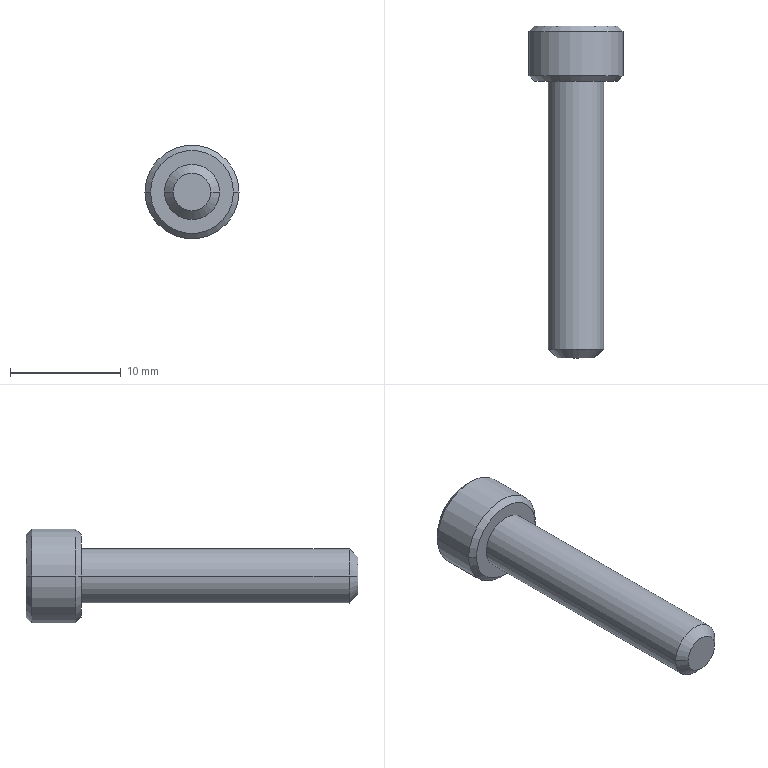Part | STEP file | BB62-M5-25L-1 | 1 solid | 27 faces | box 8.5 x 30 x 8.5 mm | volume 722.372 mm3 | plane 15 | cone 8 | cylinder 4 | commonest cylinder face diameters 5 x2 8.5 x2
STEP:
#1=CARTESIAN_POINT('',(0.,1.178,0.));
#2=VERTEX_POINT('',#1);
#3=CARTESIAN_POINT('',(2.29,2.5,0.));
#4=VERTEX_POINT('',#3);
#5=CARTESIAN_POINT('',(0.,1.178,0.));
#6=DIRECTION('',(0.866,0.5,0.));
#7=VECTOR('',#6,1000.);
#8=LINE('',#5,#7);
#9=EDGE_CURVE('',#2,#4,#8,.T.);
#10=ORIENTED_EDGE('',*,*,#9,.F.);
#11=CARTESIAN_POINT('',(-2.29,2.5,0.));
#12=VERTEX_POINT('',#11);
#13=CARTESIAN_POINT('',(0.,1.178,0.));
#14=DIRECTION('',(-0.866,0.5,0.));
#15=VECTOR('',#14,1000.);
#16=LINE('',#13,#15);
#17=EDGE_CURVE('',#2,#12,#16,.T.);
#18=ORIENTED_EDGE('',*,*,#17,.T.);
#19=CARTESIAN_POINT('',(-1.983,2.5,1.145));
#20=VERTEX_POINT('',#19);
#21=CARTESIAN_POINT('',(0.,2.5,0.));
#22=DIRECTION('',(0.,-1.,0.));
#23=DIRECTION('',(-1.,0.,0.));
#24=AXIS2_PLACEMENT_3D('',#21,#22,#23);
#25=CIRCLE('',#24,2.29);
#26=EDGE_CURVE('',#20,#12,#25,.T.);
#27=ORIENTED_EDGE('',*,*,#26,.F.);
#28=CARTESIAN_POINT('',(0.,2.5,2.29));
#29=VERTEX_POINT('',#28);
#30=CARTESIAN_POINT('',(0.,2.5,0.));
#31=DIRECTION('',(0.,-1.,0.));
#32=DIRECTION('',(-1.,0.,0.));
#33=AXIS2_PLACEMENT_3D('',#30,#31,#32);
#34=CIRCLE('',#33,2.29);
#35=EDGE_CURVE('',#29,#20,#34,.T.);
#36=ORIENTED_EDGE('',*,*,#35,.F.);
#37=CARTESIAN_POINT('',(1.983,2.5,1.145));
#38=VERTEX_POINT('',#37);
#39=CARTESIAN_POINT('',(0.,2.5,0.));
#40=DIRECTION('',(0.,-1.,0.));
#41=DIRECTION('',(-1.,0.,0.));
#42=AXIS2_PLACEMENT_3D('',#39,#40,#41);
#43=CIRCLE('',#42,2.29);
#44=EDGE_CURVE('',#38,#29,#43,.T.);
#45=ORIENTED_EDGE('',*,*,#44,.F.);
#46=CARTESIAN_POINT('',(0.,2.5,0.));
#47=DIRECTION('',(0.,-1.,0.));
#48=DIRECTION('',(-1.,0.,0.));
#49=AXIS2_PLACEMENT_3D('',#46,#47,#48);
#50=CIRCLE('',#49,2.29);
#51=EDGE_CURVE('',#4,#38,#50,.T.);
#52=ORIENTED_EDGE('',*,*,#51,.F.);
#53=EDGE_LOOP('',(#10,#18,#27,#36,#45,#52));
#54=FACE_OUTER_BOUND('',#53,.T.);
#55=CARTESIAN_POINT('',(0.,1001.178,0.));
#56=DIRECTION('',(0.,1.,0.));
#57=DIRECTION('',(1.,0.,0.));
#58=AXIS2_PLACEMENT_3D('',#55,#56,#57);
#59=CONICAL_SURFACE('',#58,1732.051,1.047);
#60=ADVANCED_FACE('',(#54),#59,.F.);
#61=CARTESIAN_POINT('',(1.7,-25.,0.));
#62=VERTEX_POINT('',#61);
#63=CARTESIAN_POINT('',(-1.7,-25.,0.));
#64=VERTEX_POINT('',#63);
#65=CARTESIAN_POINT('',(0.,-25.,0.));
#66=DIRECTION('',(0.,1.,0.));
#67=DIRECTION('',(1.,0.,0.));
#68=AXIS2_PLACEMENT_3D('',#65,#66,#67);
#69=CIRCLE('',#68,1.7);
#70=EDGE_CURVE('',#62,#64,#69,.T.);
#71=ORIENTED_EDGE('',*,*,#70,.T.);
#72=CARTESIAN_POINT('',(-2.5,-24.2,0.));
#73=VERTEX_POINT('',#72);
#74=CARTESIAN_POINT('',(-1.7,-25.,0.));
#75=DIRECTION('',(-0.7071,0.7071,0.));
#76=VECTOR('',#75,1000.);
#77=LINE('',#74,#76);
#78=EDGE_CURVE('',#64,#73,#77,.T.);
#79=ORIENTED_EDGE('',*,*,#78,.T.);
#80=CARTESIAN_POINT('',(2.5,-24.2,0.));
#81=VERTEX_POINT('',#80);
#82=CARTESIAN_POINT('',(0.,-24.2,0.));
#83=DIRECTION('',(0.,-1.,0.));
#84=DIRECTION('',(-1.,0.,0.));
#85=AXIS2_PLACEMENT_3D('',#82,#83,#84);
#86=CIRCLE('',#85,2.5);
#87=EDGE_CURVE('',#73,#81,#86,.T.);
#88=ORIENTED_EDGE('',*,*,#87,.T.);
#89=CARTESIAN_POINT('',(1.7,-25.,0.));
#90=DIRECTION('',(0.7071,0.7071,0.));
#91=VECTOR('',#90,1000.);
#92=LINE('',#89,#91);
#93=EDGE_CURVE('',#62,#81,#92,.T.);
#94=ORIENTED_EDGE('',*,*,#93,.F.);
#95=EDGE_LOOP('',(#71,#79,#88,#94));
#96=FACE_OUTER_BOUND('',#95,.T.);
#97=CARTESIAN_POINT('',(0.,-25.,0.));
#98=DIRECTION('',(0.,1.,0.));
#99=DIRECTION('',(1.,0.,0.));
#100=AXIS2_PLACEMENT_3D('',#97,#98,#99);
#101=CONICAL_SURFACE('',#100,1.7,0.7854);
#102=ADVANCED_FACE('',(#96),#101,.T.);
#103=ORIENTED_EDGE('',*,*,#87,.F.);
#104=CARTESIAN_POINT('',(-2.5,0.,0.));
#105=VERTEX_POINT('',#104);
#106=CARTESIAN_POINT('',(-2.5,-24.2,0.));
#107=DIRECTION('',(0.,1.,0.));
#108=VECTOR('',#107,1000.);
#109=LINE('',#106,#108);
#110=EDGE_CURVE('',#73,#105,#109,.T.);
#111=ORIENTED_EDGE('',*,*,#110,.T.);
#112=CARTESIAN_POINT('',(2.5,0.,0.));
#113=VERTEX_POINT('',#112);
#114=CARTESIAN_POINT('',(0.,0.,0.));
#115=DIRECTION('',(0.,-1.,0.));
#116=DIRECTION('',(-1.,0.,0.));
#117=AXIS2_PLACEMENT_3D('',#114,#115,#116);
#118=CIRCLE('',#117,2.5);
#119=EDGE_CURVE('',#105,#113,#118,.T.);
#120=ORIENTED_EDGE('',*,*,#119,.T.);
#121=CARTESIAN_POINT('',(2.5,-24.2,0.));
#122=DIRECTION('',(0.,1.,0.));
#123=VECTOR('',#122,1000.);
#124=LINE('',#121,#123);
#125=EDGE_CURVE('',#81,#113,#124,.T.);
#126=ORIENTED_EDGE('',*,*,#125,.F.);
#127=EDGE_LOOP('',(#103,#111,#120,#126));
#128=FACE_OUTER_BOUND('',#127,.T.);
#129=CARTESIAN_POINT('',(0.,-24.2,0.));
#130=DIRECTION('',(0.,1.,0.));
#131=DIRECTION('',(1.,0.,0.));
#132=AXIS2_PLACEMENT_3D('',#129,#130,#131);
#133=CYLINDRICAL_SURFACE('',#132,2.5);
#134=ADVANCED_FACE('',(#128),#133,.T.);
#135=CARTESIAN_POINT('',(-3.75,5.,0.));
#136=VERTEX_POINT('',#135);
#137=CARTESIAN_POINT('',(3.75,5.,0.));
#138=VERTEX_POINT('',#137);
#139=CARTESIAN_POINT('',(0.,5.,0.));
#140=DIRECTION('',(0.,-1.,0.));
#141=DIRECTION('',(-1.,0.,0.));
#142=AXIS2_PLACEMENT_3D('',#139,#140,#141);
#143=CIRCLE('',#142,3.75);
#144=EDGE_CURVE('',#136,#138,#143,.T.);
#145=ORIENTED_EDGE('',*,*,#144,.T.);
#146=CARTESIAN_POINT('',(4.25,4.5,0.));
#147=VERTEX_POINT('',#146);
#148=CARTESIAN_POINT('',(4.25,4.5,0.));
#149=DIRECTION('',(0.7071,-0.7071,0.));
#150=VECTOR('',#149,1000.);
#151=LINE('',#148,#150);
#152=EDGE_CURVE('',#138,#147,#151,.T.);
#153=ORIENTED_EDGE('',*,*,#152,.T.);
#154=CARTESIAN_POINT('',(-4.25,4.5,0.));
#155=VERTEX_POINT('',#154);
#156=CARTESIAN_POINT('',(0.,4.5,0.));
#157=DIRECTION('',(0.,-1.,0.));
#158=DIRECTION('',(-1.,0.,0.));
#159=AXIS2_PLACEMENT_3D('',#156,#157,#158);
#160=CIRCLE('',#159,4.25);
#161=EDGE_CURVE('',#155,#147,#160,.T.);
#162=ORIENTED_EDGE('',*,*,#161,.F.);
#163=CARTESIAN_POINT('',(-4.25,4.5,0.));
#164=DIRECTION('',(-0.7071,-0.7071,0.));
#165=VECTOR('',#164,1000.);
#166=LINE('',#163,#165);
#167=EDGE_CURVE('',#136,#155,#166,.T.);
#168=ORIENTED_EDGE('',*,*,#167,.F.);
#169=EDGE_LOOP('',(#145,#153,#162,#168));
#170=FACE_OUTER_BOUND('',#169,.T.);
#171=CARTESIAN_POINT('',(0.,4.5,0.));
#172=DIRECTION('',(0.,-1.,0.));
#173=DIRECTION('',(-1.,0.,0.));
#174=AXIS2_PLACEMENT_3D('',#171,#172,#173);
#175=CONICAL_SURFACE('',#174,4.25,0.7854);
#176=ADVANCED_FACE('',(#170),#175,.T.);
#177=ORIENTED_EDGE('',*,*,#161,.T.);
#178=CARTESIAN_POINT('',(4.25,0.5,0.));
#179=VERTEX_POINT('',#178);
#180=CARTESIAN_POINT('',(4.25,1.62,0.));
#181=DIRECTION('',(0.,-1.,0.));
#182=VECTOR('',#181,1000.);
#183=LINE('',#180,#182);
#184=EDGE_CURVE('',#147,#179,#183,.T.);
#185=ORIENTED_EDGE('',*,*,#184,.T.);
#186=CARTESIAN_POINT('',(-4.25,0.5,0.));
#187=VERTEX_POINT('',#186);
#188=CARTESIAN_POINT('',(0.,0.5,0.));
#189=DIRECTION('',(0.,-1.,0.));
#190=DIRECTION('',(-1.,0.,0.));
#191=AXIS2_PLACEMENT_3D('',#188,#189,#190);
#192=CIRCLE('',#191,4.25);
#193=EDGE_CURVE('',#187,#179,#192,.T.);
#194=ORIENTED_EDGE('',*,*,#193,.F.);
#195=CARTESIAN_POINT('',(-4.25,1.62,0.));
#196=DIRECTION('',(0.,-1.,0.));
#197=VECTOR('',#196,1000.);
#198=LINE('',#195,#197);
#199=EDGE_CURVE('',#155,#187,#198,.T.);
#200=ORIENTED_EDGE('',*,*,#199,.F.);
#201=EDGE_LOOP('',(#177,#185,#194,#200));
#202=FACE_OUTER_BOUND('',#201,.T.);
#203=CARTESIAN_POINT('',(0.,1.62,0.));
#204=DIRECTION('',(0.,-1.,0.));
#205=DIRECTION('',(-1.,0.,0.));
#206=AXIS2_PLACEMENT_3D('',#203,#204,#205);
#207=CYLINDRICAL_SURFACE('',#206,4.25);
#208=ADVANCED_FACE('',(#202),#207,.T.);
#209=CARTESIAN_POINT('',(-3.75,0.,0.));
#210=VERTEX_POINT('',#209);
#211=CARTESIAN_POINT('',(3.75,0.,0.));
#212=VERTEX_POINT('',#211);
#213=CARTESIAN_POINT('',(0.,0.,0.));
#214=DIRECTION('',(0.,-1.,0.));
#215=DIRECTION('',(-1.,0.,0.));
#216=AXIS2_PLACEMENT_3D('',#213,#214,#215);
#217=CIRCLE('',#216,3.75);
#218=EDGE_CURVE('',#210,#212,#217,.T.);
#219=ORIENTED_EDGE('',*,*,#218,.F.);
#220=CARTESIAN_POINT('',(-3.75,0.,0.));
#221=DIRECTION('',(-0.7071,0.7071,0.));
#222=VECTOR('',#221,1000.);
#223=LINE('',#220,#222);
#224=EDGE_CURVE('',#210,#187,#223,.T.);
#225=ORIENTED_EDGE('',*,*,#224,.T.);
#226=ORIENTED_EDGE('',*,*,#193,.T.);
#227=CARTESIAN_POINT('',(3.75,0.,0.));
#228=DIRECTION('',(0.7071,0.7071,0.));
#229=VECTOR('',#228,1000.);
#230=LINE('',#227,#229);
#231=EDGE_CURVE('',#212,#179,#230,.T.);
#232=ORIENTED_EDGE('',*,*,#231,.F.);
#233=EDGE_LOOP('',(#219,#225,#226,#232));
#234=FACE_OUTER_BOUND('',#233,.T.);
#235=CARTESIAN_POINT('',(0.,0.,0.));
#236=DIRECTION('',(0.,1.,0.));
#237=DIRECTION('',(1.,0.,0.));
#238=AXIS2_PLACEMENT_3D('',#235,#236,#237);
#239=CONICAL_SURFACE('',#238,3.75,0.7854);
#240=ADVANCED_FACE('',(#234),#239,.T.);
#241=ORIENTED_EDGE('',*,*,#144,.F.);
#242=CARTESIAN_POINT('',(0.,5.,0.));
#243=DIRECTION('',(0.,-1.,0.));
#244=DIRECTION('',(-1.,0.,0.));
#245=AXIS2_PLACEMENT_3D('',#242,#243,#244);
#246=CIRCLE('',#245,3.75);
#247=EDGE_CURVE('',#138,#136,#246,.T.);
#248=ORIENTED_EDGE('',*,*,#247,.F.);
#249=EDGE_LOOP('',(#241,#248));
#250=FACE_OUTER_BOUND('',#249,.T.);
#251=CARTESIAN_POINT('',(0.,5.,-2.29));
#252=VERTEX_POINT('',#251);
#253=CARTESIAN_POINT('',(-1.983,5.,-1.145));
#254=VERTEX_POINT('',#253);
#255=CARTESIAN_POINT('',(0.,5.,-2.29));
#256=DIRECTION('',(-0.866,0.,0.5));
#257=VECTOR('',#256,1000.);
#258=LINE('',#255,#257);
#259=EDGE_CURVE('',#252,#254,#258,.T.);
#260=ORIENTED_EDGE('',*,*,#259,.F.);
#261=CARTESIAN_POINT('',(1.983,5.,-1.145));
#262=VERTEX_POINT('',#261);
#263=CARTESIAN_POINT('',(1.983,5.,-1.145));
#264=DIRECTION('',(-0.866,0.,-0.5));
#265=VECTOR('',#264,1000.);
#266=LINE('',#263,#265);
#267=EDGE_CURVE('',#262,#252,#266,.T.);
#268=ORIENTED_EDGE('',*,*,#267,.F.);
#269=CARTESIAN_POINT('',(1.983,5.,1.145));
#270=VERTEX_POINT('',#269);
#271=CARTESIAN_POINT('',(1.983,5.,1.145));
#272=DIRECTION('',(0.,0.,-1.));
#273=VECTOR('',#272,1000.);
#274=LINE('',#271,#273);
#275=EDGE_CURVE('',#270,#262,#274,.T.);
#276=ORIENTED_EDGE('',*,*,#275,.F.);
#277=CARTESIAN_POINT('',(0.,5.,2.29));
#278=VERTEX_POINT('',#277);
#279=CARTESIAN_POINT('',(0.,5.,2.29));
#280=DIRECTION('',(0.866,0.,-0.5));
#281=VECTOR('',#280,1000.);
#282=LINE('',#279,#281);
#283=EDGE_CURVE('',#278,#270,#282,.T.);
#284=ORIENTED_EDGE('',*,*,#283,.F.);
#285=CARTESIAN_POINT('',(-1.983,5.,1.145));
#286=VERTEX_POINT('',#285);
#287=CARTESIAN_POINT('',(-1.983,5.,1.145));
#288=DIRECTION('',(0.866,0.,0.5));
#289=VECTOR('',#288,1000.);
#290=LINE('',#287,#289);
#291=EDGE_CURVE('',#286,#278,#290,.T.);
#292=ORIENTED_EDGE('',*,*,#291,.F.);
#293=CARTESIAN_POINT('',(-1.983,5.,-1.145));
#294=DIRECTION('',(0.,0.,1.));
#295=VECTOR('',#294,1000.);
#296=LINE('',#293,#295);
#297=EDGE_CURVE('',#254,#286,#296,.T.);
#298=ORIENTED_EDGE('',*,*,#297,.F.);
#299=EDGE_LOOP('',(#260,#268,#276,#284,#292,#298));
#300=FACE_BOUND('',#299,.T.);
#301=CARTESIAN_POINT('',(3.75,5.,0.));
#302=DIRECTION('',(0.,1.,0.));
#303=DIRECTION('',(1.,0.,0.));
#304=AXIS2_PLACEMENT_3D('',#301,#302,#303);
#305=PLANE('',#304);
#306=ADVANCED_FACE('',(#250,#300),#305,.T.);
#307=CARTESIAN_POINT('',(0.,0.,0.));
#308=DIRECTION('',(0.,-1.,0.));
#309=DIRECTION('',(-1.,0.,0.));
#310=AXIS2_PLACEMENT_3D('',#307,#308,#309);
#311=CIRCLE('',#310,2.5);
#312=EDGE_CURVE('',#113,#105,#311,.T.);
#313=ORIENTED_EDGE('',*,*,#312,.F.);
#314=ORIENTED_EDGE('',*,*,#119,.F.);
#315=EDGE_LOOP('',(#313,#314));
#316=FACE_BOUND('',#315,.T.);
#317=CARTESIAN_POINT('',(0.,0.,0.));
#318=DIRECTION('',(0.,-1.,0.));
#319=DIRECTION('',(-1.,0.,0.));
#320=AXIS2_PLACEMENT_3D('',#317,#318,#319);
#321=CIRCLE('',#320,3.75);
#322=EDGE_CURVE('',#212,#210,#321,.T.);
#323=ORIENTED_EDGE('',*,*,#322,.T.);
#324=ORIENTED_EDGE('',*,*,#218,.T.);
#325=EDGE_LOOP('',(#323,#324));
#326=FACE_OUTER_BOUND('',#325,.T.);
#327=CARTESIAN_POINT('',(0.,0.,0.));
#328=DIRECTION('',(0.,-1.,0.));
#329=DIRECTION('',(-1.,0.,0.));
#330=AXIS2_PLACEMENT_3D('',#327,#328,#329);
#331=PLANE('',#330);
#332=ADVANCED_FACE('',(#316,#326),#331,.T.);
#333=ORIENTED_EDGE('',*,*,#224,.F.);
#334=ORIENTED_EDGE('',*,*,#322,.F.);
#335=ORIENTED_EDGE('',*,*,#231,.T.);
#336=CARTESIAN_POINT('',(0.,0.5,0.));
#337=DIRECTION('',(0.,-1.,0.));
#338=DIRECTION('',(-1.,0.,0.));
#339=AXIS2_PLACEMENT_3D('',#336,#337,#338);
#340=CIRCLE('',#339,4.25);
#341=EDGE_CURVE('',#179,#187,#340,.T.);
#342=ORIENTED_EDGE('',*,*,#341,.T.);
#343=EDGE_LOOP('',(#333,#334,#335,#342));
#344=FACE_OUTER_BOUND('',#343,.T.);
#345=CARTESIAN_POINT('',(0.,0.,0.));
#346=DIRECTION('',(0.,1.,0.));
#347=DIRECTION('',(1.,0.,0.));
#348=AXIS2_PLACEMENT_3D('',#345,#346,#347);
#349=CONICAL_SURFACE('',#348,3.75,0.7854);
#350=ADVANCED_FACE('',(#344),#349,.T.);
#351=ORIENTED_EDGE('',*,*,#184,.F.);
#352=CARTESIAN_POINT('',(0.,4.5,0.));
#353=DIRECTION('',(0.,-1.,0.));
#354=DIRECTION('',(-1.,0.,0.));
#355=AXIS2_PLACEMENT_3D('',#352,#353,#354);
#356=CIRCLE('',#355,4.25);
#357=EDGE_CURVE('',#147,#155,#356,.T.);
#358=ORIENTED_EDGE('',*,*,#357,.T.);
#359=ORIENTED_EDGE('',*,*,#199,.T.);
#360=ORIENTED_EDGE('',*,*,#341,.F.);
#361=EDGE_LOOP('',(#351,#358,#359,#360));
#362=FACE_OUTER_BOUND('',#361,.T.);
#363=CARTESIAN_POINT('',(0.,1.62,0.));
#364=DIRECTION('',(0.,-1.,0.));
#365=DIRECTION('',(-1.,0.,0.));
#366=AXIS2_PLACEMENT_3D('',#363,#364,#365);
#367=CYLINDRICAL_SURFACE('',#366,4.25);
#368=ADVANCED_FACE('',(#362),#367,.T.);
#369=ORIENTED_EDGE('',*,*,#152,.F.);
#370=ORIENTED_EDGE('',*,*,#247,.T.);
#371=ORIENTED_EDGE('',*,*,#167,.T.);
#372=ORIENTED_EDGE('',*,*,#357,.F.);
#373=EDGE_LOOP('',(#369,#370,#371,#372));
#374=FACE_OUTER_BOUND('',#373,.T.);
#375=CARTESIAN_POINT('',(0.,4.5,0.));
#376=DIRECTION('',(0.,-1.,0.));
#377=DIRECTION('',(-1.,0.,0.));
#378=AXIS2_PLACEMENT_3D('',#375,#376,#377);
#379=CONICAL_SURFACE('',#378,4.25,0.7854);
#380=ADVANCED_FACE('',(#374),#379,.T.);
#381=ORIENTED_EDGE('',*,*,#110,.F.);
#382=CARTESIAN_POINT('',(0.,-24.2,0.));
#383=DIRECTION('',(0.,-1.,0.));
#384=DIRECTION('',(-1.,0.,0.));
#385=AXIS2_PLACEMENT_3D('',#382,#383,#384);
#386=CIRCLE('',#385,2.5);
#387=EDGE_CURVE('',#81,#73,#386,.T.);
#388=ORIENTED_EDGE('',*,*,#387,.F.);
#389=ORIENTED_EDGE('',*,*,#125,.T.);
#390=ORIENTED_EDGE('',*,*,#312,.T.);
#391=EDGE_LOOP('',(#381,#388,#389,#390));
#392=FACE_OUTER_BOUND('',#391,.T.);
#393=CARTESIAN_POINT('',(0.,-24.2,0.));
#394=DIRECTION('',(0.,1.,0.));
#395=DIRECTION('',(1.,0.,0.));
#396=AXIS2_PLACEMENT_3D('',#393,#394,#395);
#397=CYLINDRICAL_SURFACE('',#396,2.5);
#398=ADVANCED_FACE('',(#392),#397,.T.);
#399=ORIENTED_EDGE('',*,*,#70,.F.);
#400=CARTESIAN_POINT('',(0.,-25.,0.));
#401=DIRECTION('',(0.,1.,0.));
#402=DIRECTION('',(1.,0.,0.));
#403=AXIS2_PLACEMENT_3D('',#400,#401,#402);
#404=CIRCLE('',#403,1.7);
#405=EDGE_CURVE('',#64,#62,#404,.T.);
#406=ORIENTED_EDGE('',*,*,#405,.F.);
#407=EDGE_LOOP('',(#399,#406));
#408=FACE_OUTER_BOUND('',#407,.T.);
#409=CARTESIAN_POINT('',(0.,-25.,0.));
#410=DIRECTION('',(0.,-1.,0.));
#411=DIRECTION('',(-1.,0.,0.));
#412=AXIS2_PLACEMENT_3D('',#409,#410,#411);
#413=PLANE('',#412);
#414=ADVANCED_FACE('',(#408),#413,.T.);
#415=ORIENTED_EDGE('',*,*,#78,.F.);
#416=ORIENTED_EDGE('',*,*,#405,.T.);
#417=ORIENTED_EDGE('',*,*,#93,.T.);
#418=ORIENTED_EDGE('',*,*,#387,.T.);
#419=EDGE_LOOP('',(#415,#416,#417,#418));
#420=FACE_OUTER_BOUND('',#419,.T.);
#421=CARTESIAN_POINT('',(0.,-25.,0.));
#422=DIRECTION('',(0.,1.,0.));
#423=DIRECTION('',(1.,0.,0.));
#424=AXIS2_PLACEMENT_3D('',#421,#422,#423);
#425=CONICAL_SURFACE('',#424,1.7,0.7854);
#426=ADVANCED_FACE('',(#420),#425,.T.);
#427=CARTESIAN_POINT('',(1.983,2.5,-1.145));
#428=VERTEX_POINT('',#427);
#429=CARTESIAN_POINT('',(0.,2.5,-2.29));
#430=VERTEX_POINT('',#429);
#431=CARTESIAN_POINT('',(1.983,2.5,-1.145));
#432=DIRECTION('',(-0.866,0.,-0.5));
#433=VECTOR('',#432,1000.);
#434=LINE('',#431,#433);
#435=EDGE_CURVE('',#428,#430,#434,.T.);
#436=ORIENTED_EDGE('',*,*,#435,.F.);
#437=CARTESIAN_POINT('',(1.983,5.,-1.145));
#438=DIRECTION('',(0.,-1.,0.));
#439=VECTOR('',#438,1000.);
#440=LINE('',#437,#439);
#441=EDGE_CURVE('',#262,#428,#440,.T.);
#442=ORIENTED_EDGE('',*,*,#441,.F.);
#443=ORIENTED_EDGE('',*,*,#267,.T.);
#444=CARTESIAN_POINT('',(0.,5.,-2.29));
#445=DIRECTION('',(0.,-1.,0.));
#446=VECTOR('',#445,1000.);
#447=LINE('',#444,#446);
#448=EDGE_CURVE('',#252,#430,#447,.T.);
#449=ORIENTED_EDGE('',*,*,#448,.T.);
#450=EDGE_LOOP('',(#436,#442,#443,#449));
#451=FACE_OUTER_BOUND('',#450,.T.);
#452=CARTESIAN_POINT('',(1.983,5.,-1.145));
#453=DIRECTION('',(-0.5,0.,0.866));
#454=DIRECTION('',(0.866,0.,0.5));
#455=AXIS2_PLACEMENT_3D('',#452,#453,#454);
#456=PLANE('',#455);
#457=ADVANCED_FACE('',(#451),#456,.T.);
#458=CARTESIAN_POINT('',(-1.983,2.5,-1.145));
#459=VERTEX_POINT('',#458);
#460=CARTESIAN_POINT('',(0.,2.5,-2.29));
#461=DIRECTION('',(-0.866,0.,0.5));
#462=VECTOR('',#461,1000.);
#463=LINE('',#460,#462);
#464=EDGE_CURVE('',#430,#459,#463,.T.);
#465=ORIENTED_EDGE('',*,*,#464,.F.);
#466=ORIENTED_EDGE('',*,*,#448,.F.);
#467=ORIENTED_EDGE('',*,*,#259,.T.);
#468=CARTESIAN_POINT('',(-1.983,5.,-1.145));
#469=DIRECTION('',(0.,-1.,0.));
#470=VECTOR('',#469,1000.);
#471=LINE('',#468,#470);
#472=EDGE_CURVE('',#254,#459,#471,.T.);
#473=ORIENTED_EDGE('',*,*,#472,.T.);
#474=EDGE_LOOP('',(#465,#466,#467,#473));
#475=FACE_OUTER_BOUND('',#474,.T.);
#476=CARTESIAN_POINT('',(0.,5.,-2.29));
#477=DIRECTION('',(0.5,0.,0.866));
#478=DIRECTION('',(0.866,0.,-0.5));
#479=AXIS2_PLACEMENT_3D('',#476,#477,#478);
#480=PLANE('',#479);
#481=ADVANCED_FACE('',(#475),#480,.T.);
#482=CARTESIAN_POINT('',(-1.983,2.5,-1.145));
#483=DIRECTION('',(0.,0.,1.));
#484=VECTOR('',#483,1000.);
#485=LINE('',#482,#484);
#486=EDGE_CURVE('',#459,#20,#485,.T.);
#487=ORIENTED_EDGE('',*,*,#486,.F.);
#488=ORIENTED_EDGE('',*,*,#472,.F.);
#489=ORIENTED_EDGE('',*,*,#297,.T.);
#490=CARTESIAN_POINT('',(-1.983,5.,1.145));
#491=DIRECTION('',(0.,-1.,0.));
#492=VECTOR('',#491,1000.);
#493=LINE('',#490,#492);
#494=EDGE_CURVE('',#286,#20,#493,.T.);
#495=ORIENTED_EDGE('',*,*,#494,.T.);
#496=EDGE_LOOP('',(#487,#488,#489,#495));
#497=FACE_OUTER_BOUND('',#496,.T.);
#498=CARTESIAN_POINT('',(-1.983,5.,-1.145));
#499=DIRECTION('',(1.,0.,0.));
#500=DIRECTION('',(0.,0.,-1.));
#501=AXIS2_PLACEMENT_3D('',#498,#499,#500);
#502=PLANE('',#501);
#503=ADVANCED_FACE('',(#497),#502,.T.);
#504=CARTESIAN_POINT('',(-1.983,2.5,1.145));
#505=DIRECTION('',(0.866,0.,0.5));
#506=VECTOR('',#505,1000.);
#507=LINE('',#504,#506);
#508=EDGE_CURVE('',#20,#29,#507,.T.);
#509=ORIENTED_EDGE('',*,*,#508,.F.);
#510=ORIENTED_EDGE('',*,*,#494,.F.);
#511=ORIENTED_EDGE('',*,*,#291,.T.);
#512=CARTESIAN_POINT('',(0.,5.,2.29));
#513=DIRECTION('',(0.,-1.,0.));
#514=VECTOR('',#513,1000.);
#515=LINE('',#512,#514);
#516=EDGE_CURVE('',#278,#29,#515,.T.);
#517=ORIENTED_EDGE('',*,*,#516,.T.);
#518=EDGE_LOOP('',(#509,#510,#511,#517));
#519=FACE_OUTER_BOUND('',#518,.T.);
#520=CARTESIAN_POINT('',(-1.983,5.,1.145));
#521=DIRECTION('',(0.5,0.,-0.866));
#522=DIRECTION('',(-0.866,0.,-0.5));
#523=AXIS2_PLACEMENT_3D('',#520,#521,#522);
#524=PLANE('',#523);
#525=ADVANCED_FACE('',(#519),#524,.T.);
#526=CARTESIAN_POINT('',(0.,2.5,2.29));
#527=DIRECTION('',(0.866,0.,-0.5));
#528=VECTOR('',#527,1000.);
#529=LINE('',#526,#528);
#530=EDGE_CURVE('',#29,#38,#529,.T.);
#531=ORIENTED_EDGE('',*,*,#530,.F.);
#532=ORIENTED_EDGE('',*,*,#516,.F.);
#533=ORIENTED_EDGE('',*,*,#283,.T.);
#534=CARTESIAN_POINT('',(1.983,5.,1.145));
#535=DIRECTION('',(0.,-1.,0.));
#536=VECTOR('',#535,1000.);
#537=LINE('',#534,#536);
#538=EDGE_CURVE('',#270,#38,#537,.T.);
#539=ORIENTED_EDGE('',*,*,#538,.T.);
#540=EDGE_LOOP('',(#531,#532,#533,#539));
#541=FACE_OUTER_BOUND('',#540,.T.);
#542=CARTESIAN_POINT('',(0.,5.,2.29));
#543=DIRECTION('',(-0.5,0.,-0.866));
#544=DIRECTION('',(-0.866,0.,0.5));
#545=AXIS2_PLACEMENT_3D('',#542,#543,#544);
#546=PLANE('',#545);
#547=ADVANCED_FACE('',(#541),#546,.T.);
#548=CARTESIAN_POINT('',(1.983,2.5,1.145));
#549=DIRECTION('',(0.,0.,-1.));
#550=VECTOR('',#549,1000.);
#551=LINE('',#548,#550);
#552=EDGE_CURVE('',#38,#428,#551,.T.);
#553=ORIENTED_EDGE('',*,*,#552,.F.);
#554=ORIENTED_EDGE('',*,*,#538,.F.);
#555=ORIENTED_EDGE('',*,*,#275,.T.);
#556=ORIENTED_EDGE('',*,*,#441,.T.);
#557=EDGE_LOOP('',(#553,#554,#555,#556));
#558=FACE_OUTER_BOUND('',#557,.T.);
#559=CARTESIAN_POINT('',(1.983,5.,1.145));
#560=DIRECTION('',(-1.,0.,0.));
#561=DIRECTION('',(0.,0.,1.));
#562=AXIS2_PLACEMENT_3D('',#559,#560,#561);
#563=PLANE('',#562);
#564=ADVANCED_FACE('',(#558),#563,.T.);
#565=ORIENTED_EDGE('',*,*,#435,.T.);
#566=CARTESIAN_POINT('',(0.,2.5,0.));
#567=DIRECTION('',(0.,-1.,0.));
#568=DIRECTION('',(-1.,0.,0.));
#569=AXIS2_PLACEMENT_3D('',#566,#567,#568);
#570=CIRCLE('',#569,2.29);
#571=EDGE_CURVE('',#430,#428,#570,.T.);
#572=ORIENTED_EDGE('',*,*,#571,.T.);
#573=EDGE_LOOP('',(#565,#572));
#574=FACE_OUTER_BOUND('',#573,.T.);
#575=CARTESIAN_POINT('',(0.,2.5,0.));
#576=DIRECTION('',(0.,1.,0.));
#577=DIRECTION('',(1.,0.,0.));
#578=AXIS2_PLACEMENT_3D('',#575,#576,#577);
#579=PLANE('',#578);
#580=ADVANCED_FACE('',(#574),#579,.F.);
#581=ORIENTED_EDGE('',*,*,#552,.T.);
#582=CARTESIAN_POINT('',(0.,2.5,0.));
#583=DIRECTION('',(0.,-1.,0.));
#584=DIRECTION('',(-1.,0.,0.));
#585=AXIS2_PLACEMENT_3D('',#582,#583,#584);
#586=CIRCLE('',#585,2.29);
#587=EDGE_CURVE('',#428,#4,#586,.T.);
#588=ORIENTED_EDGE('',*,*,#587,.T.);
#589=ORIENTED_EDGE('',*,*,#51,.T.);
#590=EDGE_LOOP('',(#581,#588,#589));
#591=FACE_OUTER_BOUND('',#590,.T.);
#592=CARTESIAN_POINT('',(0.,2.5,0.));
#593=DIRECTION('',(0.,1.,0.));
#594=DIRECTION('',(1.,0.,0.));
#595=AXIS2_PLACEMENT_3D('',#592,#593,#594);
#596=PLANE('',#595);
#597=ADVANCED_FACE('',(#591),#596,.F.);
#598=ORIENTED_EDGE('',*,*,#530,.T.);
#599=ORIENTED_EDGE('',*,*,#44,.T.);
#600=EDGE_LOOP('',(#598,#599));
#601=FACE_OUTER_BOUND('',#600,.T.);
#602=CARTESIAN_POINT('',(0.,2.5,0.));
#603=DIRECTION('',(0.,1.,0.));
#604=DIRECTION('',(1.,0.,0.));
#605=AXIS2_PLACEMENT_3D('',#602,#603,#604);
#606=PLANE('',#605);
#607=ADVANCED_FACE('',(#601),#606,.F.);
#608=ORIENTED_EDGE('',*,*,#508,.T.);
#609=ORIENTED_EDGE('',*,*,#35,.T.);
#610=EDGE_LOOP('',(#608,#609));
#611=FACE_OUTER_BOUND('',#610,.T.);
#612=CARTESIAN_POINT('',(0.,2.5,0.));
#613=DIRECTION('',(0.,1.,0.));
#614=DIRECTION('',(1.,0.,0.));
#615=AXIS2_PLACEMENT_3D('',#612,#613,#614);
#616=PLANE('',#615);
#617=ADVANCED_FACE('',(#611),#616,.F.);
#618=ORIENTED_EDGE('',*,*,#486,.T.);
#619=ORIENTED_EDGE('',*,*,#26,.T.);
#620=CARTESIAN_POINT('',(0.,2.5,0.));
#621=DIRECTION('',(0.,-1.,0.));
#622=DIRECTION('',(-1.,0.,0.));
#623=AXIS2_PLACEMENT_3D('',#620,#621,#622);
#624=CIRCLE('',#623,2.29);
#625=EDGE_CURVE('',#12,#459,#624,.T.);
#626=ORIENTED_EDGE('',*,*,#625,.T.);
#627=EDGE_LOOP('',(#618,#619,#626));
#628=FACE_OUTER_BOUND('',#627,.T.);
#629=CARTESIAN_POINT('',(0.,2.5,0.));
#630=DIRECTION('',(0.,1.,0.));
#631=DIRECTION('',(1.,0.,0.));
#632=AXIS2_PLACEMENT_3D('',#629,#630,#631);
#633=PLANE('',#632);
#634=ADVANCED_FACE('',(#628),#633,.F.);
#635=ORIENTED_EDGE('',*,*,#464,.T.);
#636=CARTESIAN_POINT('',(0.,2.5,0.));
#637=DIRECTION('',(0.,-1.,0.));
#638=DIRECTION('',(-1.,0.,0.));
#639=AXIS2_PLACEMENT_3D('',#636,#637,#638);
#640=CIRCLE('',#639,2.29);
#641=EDGE_CURVE('',#459,#430,#640,.T.);
#642=ORIENTED_EDGE('',*,*,#641,.T.);
#643=EDGE_LOOP('',(#635,#642));
#644=FACE_OUTER_BOUND('',#643,.T.);
#645=CARTESIAN_POINT('',(0.,2.5,0.));
#646=DIRECTION('',(0.,1.,0.));
#647=DIRECTION('',(1.,0.,0.));
#648=AXIS2_PLACEMENT_3D('',#645,#646,#647);
#649=PLANE('',#648);
#650=ADVANCED_FACE('',(#644),#649,.F.);
#651=ORIENTED_EDGE('',*,*,#17,.F.);
#652=ORIENTED_EDGE('',*,*,#9,.T.);
#653=ORIENTED_EDGE('',*,*,#587,.F.);
#654=ORIENTED_EDGE('',*,*,#571,.F.);
#655=ORIENTED_EDGE('',*,*,#641,.F.);
#656=ORIENTED_EDGE('',*,*,#625,.F.);
#657=EDGE_LOOP('',(#651,#652,#653,#654,#655,#656));
#658=FACE_OUTER_BOUND('',#657,.T.);
#659=CARTESIAN_POINT('',(0.,1001.178,0.));
#660=DIRECTION('',(0.,1.,0.));
#661=DIRECTION('',(1.,0.,0.));
#662=AXIS2_PLACEMENT_3D('',#659,#660,#661);
#663=CONICAL_SURFACE('',#662,1732.051,1.047);
#664=ADVANCED_FACE('',(#658),#663,.F.);
#665=CLOSED_SHELL('',(#60,#102,#134,#176,#208,#240,#306,#332,#350,#368,#380,#398,#414,#426,#457,#481,#503,#525,#547,#564,#580,#597,#607,#617,#634,#650,#664));
#666=MANIFOLD_SOLID_BREP('',#665);
#667=CARTESIAN_POINT('',(0.,0.,0.));
#668=DIRECTION('',(0.,0.,1.));
#669=DIRECTION('',(1.,0.,0.));
#670=AXIS2_PLACEMENT_3D('',#667,#668,#669);
#671=(LENGTH_UNIT()NAMED_UNIT(*)SI_UNIT(.MILLI.,.METRE.));
#672=UNCERTAINTY_MEASURE_WITH_UNIT(LENGTH_MEASURE(0.00001),#671,'','');
#673=(NAMED_UNIT(*)PLANE_ANGLE_UNIT()SI_UNIT($,.RADIAN.));
#674=(NAMED_UNIT(*)SI_UNIT($,.STERADIAN.)SOLID_ANGLE_UNIT());
#675=(GEOMETRIC_REPRESENTATION_CONTEXT(3)GLOBAL_UNCERTAINTY_ASSIGNED_CONTEXT((#672))GLOBAL_UNIT_ASSIGNED_CONTEXT((#671,#673,#674))REPRESENTATION_CONTEXT('',''));
#676=ADVANCED_BREP_SHAPE_REPRESENTATION('',(#666,#670),#675);